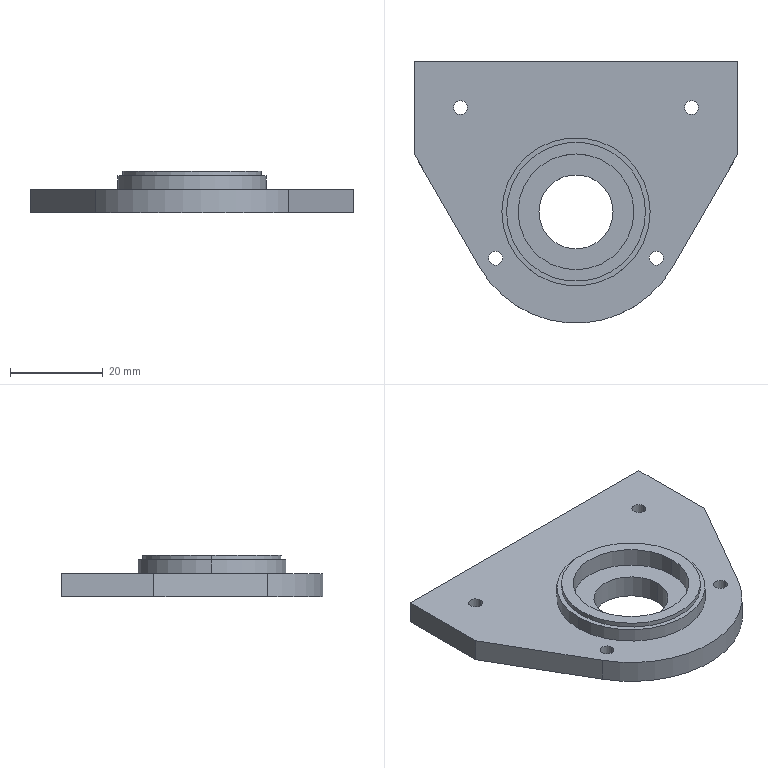Part | SolidWorks | features BaseBody 1 | 1 solid | 39 faces | box 69.859 x 56.5 x 9 mm | volume 15464 mm3 | cylinder 25 | plane 14 | commonest cylinder face diameters 3 x8 5 x8 16 x2 25 x2 30 x2 32 x2
STEP:
#1=CARTESIAN_POINT('',(-22.43,22.5,2.5));
#2=VERTEX_POINT('',#1);
#3=CARTESIAN_POINT('',(-27.43,22.5,2.5));
#4=VERTEX_POINT('',#3);
#5=CARTESIAN_POINT('',(-24.93,22.5,2.5));
#6=DIRECTION('',(0.,0.,1.));
#7=DIRECTION('',(1.,0.,0.));
#8=AXIS2_PLACEMENT_3D('',#5,#6,#7);
#9=CIRCLE('',#8,2.5);
#10=EDGE_CURVE('',#2,#4,#9,.T.);
#11=ORIENTED_EDGE('',*,*,#10,.T.);
#12=CARTESIAN_POINT('',(-27.43,22.5,0.));
#13=VERTEX_POINT('',#12);
#14=CARTESIAN_POINT('',(-27.43,22.5,0.));
#15=DIRECTION('',(0.,0.,-1.));
#16=VECTOR('',#15,1000.);
#17=LINE('',#14,#16);
#18=EDGE_CURVE('',#4,#13,#17,.T.);
#19=ORIENTED_EDGE('',*,*,#18,.T.);
#20=CARTESIAN_POINT('',(-22.43,22.5,0.));
#21=VERTEX_POINT('',#20);
#22=CARTESIAN_POINT('',(-24.93,22.5,0.));
#23=DIRECTION('',(0.,0.,1.));
#24=DIRECTION('',(1.,0.,0.));
#25=AXIS2_PLACEMENT_3D('',#22,#23,#24);
#26=CIRCLE('',#25,2.5);
#27=EDGE_CURVE('',#21,#13,#26,.T.);
#28=ORIENTED_EDGE('',*,*,#27,.F.);
#29=CARTESIAN_POINT('',(-22.43,22.5,0.));
#30=DIRECTION('',(0.,0.,-1.));
#31=VECTOR('',#30,1000.);
#32=LINE('',#29,#31);
#33=EDGE_CURVE('',#2,#21,#32,.T.);
#34=ORIENTED_EDGE('',*,*,#33,.F.);
#35=EDGE_LOOP('',(#11,#19,#28,#34));
#36=FACE_OUTER_BOUND('',#35,.T.);
#37=CARTESIAN_POINT('',(-24.93,22.5,0.));
#38=DIRECTION('',(0.,0.,-1.));
#39=DIRECTION('',(1.,0.,0.));
#40=AXIS2_PLACEMENT_3D('',#37,#38,#39);
#41=CYLINDRICAL_SURFACE('',#40,2.5);
#42=ADVANCED_FACE('',(#36),#41,.F.);
#43=CARTESIAN_POINT('',(-14.821,-10.,2.5));
#44=VERTEX_POINT('',#43);
#45=CARTESIAN_POINT('',(-19.821,-10.,2.5));
#46=VERTEX_POINT('',#45);
#47=CARTESIAN_POINT('',(-17.321,-10.,2.5));
#48=DIRECTION('',(0.,0.,1.));
#49=DIRECTION('',(1.,0.,0.));
#50=AXIS2_PLACEMENT_3D('',#47,#48,#49);
#51=CIRCLE('',#50,2.5);
#52=EDGE_CURVE('',#44,#46,#51,.T.);
#53=ORIENTED_EDGE('',*,*,#52,.T.);
#54=CARTESIAN_POINT('',(-19.821,-10.,0.));
#55=VERTEX_POINT('',#54);
#56=CARTESIAN_POINT('',(-19.821,-10.,0.));
#57=DIRECTION('',(0.,0.,-1.));
#58=VECTOR('',#57,1000.);
#59=LINE('',#56,#58);
#60=EDGE_CURVE('',#46,#55,#59,.T.);
#61=ORIENTED_EDGE('',*,*,#60,.T.);
#62=CARTESIAN_POINT('',(-14.821,-10.,0.));
#63=VERTEX_POINT('',#62);
#64=CARTESIAN_POINT('',(-17.321,-10.,0.));
#65=DIRECTION('',(0.,0.,1.));
#66=DIRECTION('',(1.,0.,0.));
#67=AXIS2_PLACEMENT_3D('',#64,#65,#66);
#68=CIRCLE('',#67,2.5);
#69=EDGE_CURVE('',#63,#55,#68,.T.);
#70=ORIENTED_EDGE('',*,*,#69,.F.);
#71=CARTESIAN_POINT('',(-14.821,-10.,0.));
#72=DIRECTION('',(0.,0.,-1.));
#73=VECTOR('',#72,1000.);
#74=LINE('',#71,#73);
#75=EDGE_CURVE('',#44,#63,#74,.T.);
#76=ORIENTED_EDGE('',*,*,#75,.F.);
#77=EDGE_LOOP('',(#53,#61,#70,#76));
#78=FACE_OUTER_BOUND('',#77,.T.);
#79=CARTESIAN_POINT('',(-17.321,-10.,0.));
#80=DIRECTION('',(0.,0.,-1.));
#81=DIRECTION('',(1.,0.,0.));
#82=AXIS2_PLACEMENT_3D('',#79,#80,#81);
#83=CYLINDRICAL_SURFACE('',#82,2.5);
#84=ADVANCED_FACE('',(#78),#83,.F.);
#85=CARTESIAN_POINT('',(19.821,-10.,2.5));
#86=VERTEX_POINT('',#85);
#87=CARTESIAN_POINT('',(14.821,-10.,2.5));
#88=VERTEX_POINT('',#87);
#89=CARTESIAN_POINT('',(17.321,-10.,2.5));
#90=DIRECTION('',(0.,0.,1.));
#91=DIRECTION('',(1.,0.,0.));
#92=AXIS2_PLACEMENT_3D('',#89,#90,#91);
#93=CIRCLE('',#92,2.5);
#94=EDGE_CURVE('',#86,#88,#93,.T.);
#95=ORIENTED_EDGE('',*,*,#94,.T.);
#96=CARTESIAN_POINT('',(14.821,-10.,0.));
#97=VERTEX_POINT('',#96);
#98=CARTESIAN_POINT('',(14.821,-10.,0.));
#99=DIRECTION('',(0.,0.,-1.));
#100=VECTOR('',#99,1000.);
#101=LINE('',#98,#100);
#102=EDGE_CURVE('',#88,#97,#101,.T.);
#103=ORIENTED_EDGE('',*,*,#102,.T.);
#104=CARTESIAN_POINT('',(19.821,-10.,0.));
#105=VERTEX_POINT('',#104);
#106=CARTESIAN_POINT('',(17.321,-10.,0.));
#107=DIRECTION('',(0.,0.,1.));
#108=DIRECTION('',(1.,0.,0.));
#109=AXIS2_PLACEMENT_3D('',#106,#107,#108);
#110=CIRCLE('',#109,2.5);
#111=EDGE_CURVE('',#105,#97,#110,.T.);
#112=ORIENTED_EDGE('',*,*,#111,.F.);
#113=CARTESIAN_POINT('',(19.821,-10.,0.));
#114=DIRECTION('',(0.,0.,-1.));
#115=VECTOR('',#114,1000.);
#116=LINE('',#113,#115);
#117=EDGE_CURVE('',#86,#105,#116,.T.);
#118=ORIENTED_EDGE('',*,*,#117,.F.);
#119=EDGE_LOOP('',(#95,#103,#112,#118));
#120=FACE_OUTER_BOUND('',#119,.T.);
#121=CARTESIAN_POINT('',(17.321,-10.,0.));
#122=DIRECTION('',(0.,0.,-1.));
#123=DIRECTION('',(1.,0.,0.));
#124=AXIS2_PLACEMENT_3D('',#121,#122,#123);
#125=CYLINDRICAL_SURFACE('',#124,2.5);
#126=ADVANCED_FACE('',(#120),#125,.F.);
#127=CARTESIAN_POINT('',(27.43,22.5,2.5));
#128=VERTEX_POINT('',#127);
#129=CARTESIAN_POINT('',(22.43,22.5,2.5));
#130=VERTEX_POINT('',#129);
#131=CARTESIAN_POINT('',(24.93,22.5,2.5));
#132=DIRECTION('',(0.,0.,1.));
#133=DIRECTION('',(1.,0.,0.));
#134=AXIS2_PLACEMENT_3D('',#131,#132,#133);
#135=CIRCLE('',#134,2.5);
#136=EDGE_CURVE('',#128,#130,#135,.T.);
#137=ORIENTED_EDGE('',*,*,#136,.T.);
#138=CARTESIAN_POINT('',(22.43,22.5,0.));
#139=VERTEX_POINT('',#138);
#140=CARTESIAN_POINT('',(22.43,22.5,0.));
#141=DIRECTION('',(0.,0.,-1.));
#142=VECTOR('',#141,1000.);
#143=LINE('',#140,#142);
#144=EDGE_CURVE('',#130,#139,#143,.T.);
#145=ORIENTED_EDGE('',*,*,#144,.T.);
#146=CARTESIAN_POINT('',(27.43,22.5,0.));
#147=VERTEX_POINT('',#146);
#148=CARTESIAN_POINT('',(24.93,22.5,0.));
#149=DIRECTION('',(0.,0.,1.));
#150=DIRECTION('',(1.,0.,0.));
#151=AXIS2_PLACEMENT_3D('',#148,#149,#150);
#152=CIRCLE('',#151,2.5);
#153=EDGE_CURVE('',#147,#139,#152,.T.);
#154=ORIENTED_EDGE('',*,*,#153,.F.);
#155=CARTESIAN_POINT('',(27.43,22.5,0.));
#156=DIRECTION('',(0.,0.,-1.));
#157=VECTOR('',#156,1000.);
#158=LINE('',#155,#157);
#159=EDGE_CURVE('',#128,#147,#158,.T.);
#160=ORIENTED_EDGE('',*,*,#159,.F.);
#161=EDGE_LOOP('',(#137,#145,#154,#160));
#162=FACE_OUTER_BOUND('',#161,.T.);
#163=CARTESIAN_POINT('',(24.93,22.5,0.));
#164=DIRECTION('',(0.,0.,-1.));
#165=DIRECTION('',(1.,0.,0.));
#166=AXIS2_PLACEMENT_3D('',#163,#164,#165);
#167=CYLINDRICAL_SURFACE('',#166,2.5);
#168=ADVANCED_FACE('',(#162),#167,.F.);
#169=CARTESIAN_POINT('',(23.43,22.5,2.5));
#170=VERTEX_POINT('',#169);
#171=CARTESIAN_POINT('',(26.43,22.5,2.5));
#172=VERTEX_POINT('',#171);
#173=CARTESIAN_POINT('',(24.93,22.5,2.5));
#174=DIRECTION('',(0.,0.,-1.));
#175=DIRECTION('',(-1.,0.,0.));
#176=AXIS2_PLACEMENT_3D('',#173,#174,#175);
#177=CIRCLE('',#176,1.5);
#178=EDGE_CURVE('',#170,#172,#177,.T.);
#179=ORIENTED_EDGE('',*,*,#178,.T.);
#180=CARTESIAN_POINT('',(26.43,22.5,5.));
#181=VERTEX_POINT('',#180);
#182=CARTESIAN_POINT('',(26.43,22.5,5.));
#183=DIRECTION('',(0.,0.,1.));
#184=VECTOR('',#183,1000.);
#185=LINE('',#182,#184);
#186=EDGE_CURVE('',#172,#181,#185,.T.);
#187=ORIENTED_EDGE('',*,*,#186,.T.);
#188=CARTESIAN_POINT('',(23.43,22.5,5.));
#189=VERTEX_POINT('',#188);
#190=CARTESIAN_POINT('',(24.93,22.5,5.));
#191=DIRECTION('',(0.,0.,-1.));
#192=DIRECTION('',(-1.,0.,0.));
#193=AXIS2_PLACEMENT_3D('',#190,#191,#192);
#194=CIRCLE('',#193,1.5);
#195=EDGE_CURVE('',#189,#181,#194,.T.);
#196=ORIENTED_EDGE('',*,*,#195,.F.);
#197=CARTESIAN_POINT('',(23.43,22.5,5.));
#198=DIRECTION('',(0.,0.,1.));
#199=VECTOR('',#198,1000.);
#200=LINE('',#197,#199);
#201=EDGE_CURVE('',#170,#189,#200,.T.);
#202=ORIENTED_EDGE('',*,*,#201,.F.);
#203=EDGE_LOOP('',(#179,#187,#196,#202));
#204=FACE_OUTER_BOUND('',#203,.T.);
#205=CARTESIAN_POINT('',(24.93,22.5,5.));
#206=DIRECTION('',(0.,0.,1.));
#207=DIRECTION('',(-1.,0.,0.));
#208=AXIS2_PLACEMENT_3D('',#205,#206,#207);
#209=CYLINDRICAL_SURFACE('',#208,1.5);
#210=ADVANCED_FACE('',(#204),#209,.F.);
#211=CARTESIAN_POINT('',(15.821,-10.,2.5));
#212=VERTEX_POINT('',#211);
#213=CARTESIAN_POINT('',(18.821,-10.,2.5));
#214=VERTEX_POINT('',#213);
#215=CARTESIAN_POINT('',(17.321,-10.,2.5));
#216=DIRECTION('',(0.,0.,-1.));
#217=DIRECTION('',(-1.,0.,0.));
#218=AXIS2_PLACEMENT_3D('',#215,#216,#217);
#219=CIRCLE('',#218,1.5);
#220=EDGE_CURVE('',#212,#214,#219,.T.);
#221=ORIENTED_EDGE('',*,*,#220,.T.);
#222=CARTESIAN_POINT('',(18.821,-10.,5.));
#223=VERTEX_POINT('',#222);
#224=CARTESIAN_POINT('',(18.821,-10.,5.));
#225=DIRECTION('',(0.,0.,1.));
#226=VECTOR('',#225,1000.);
#227=LINE('',#224,#226);
#228=EDGE_CURVE('',#214,#223,#227,.T.);
#229=ORIENTED_EDGE('',*,*,#228,.T.);
#230=CARTESIAN_POINT('',(15.821,-10.,5.));
#231=VERTEX_POINT('',#230);
#232=CARTESIAN_POINT('',(17.321,-10.,5.));
#233=DIRECTION('',(0.,0.,-1.));
#234=DIRECTION('',(-1.,0.,0.));
#235=AXIS2_PLACEMENT_3D('',#232,#233,#234);
#236=CIRCLE('',#235,1.5);
#237=EDGE_CURVE('',#231,#223,#236,.T.);
#238=ORIENTED_EDGE('',*,*,#237,.F.);
#239=CARTESIAN_POINT('',(15.821,-10.,5.));
#240=DIRECTION('',(0.,0.,1.));
#241=VECTOR('',#240,1000.);
#242=LINE('',#239,#241);
#243=EDGE_CURVE('',#212,#231,#242,.T.);
#244=ORIENTED_EDGE('',*,*,#243,.F.);
#245=EDGE_LOOP('',(#221,#229,#238,#244));
#246=FACE_OUTER_BOUND('',#245,.T.);
#247=CARTESIAN_POINT('',(17.321,-10.,5.));
#248=DIRECTION('',(0.,0.,1.));
#249=DIRECTION('',(-1.,0.,0.));
#250=AXIS2_PLACEMENT_3D('',#247,#248,#249);
#251=CYLINDRICAL_SURFACE('',#250,1.5);
#252=ADVANCED_FACE('',(#246),#251,.F.);
#253=CARTESIAN_POINT('',(-18.821,-10.,2.5));
#254=VERTEX_POINT('',#253);
#255=CARTESIAN_POINT('',(-15.821,-10.,2.5));
#256=VERTEX_POINT('',#255);
#257=CARTESIAN_POINT('',(-17.321,-10.,2.5));
#258=DIRECTION('',(0.,0.,-1.));
#259=DIRECTION('',(-1.,0.,0.));
#260=AXIS2_PLACEMENT_3D('',#257,#258,#259);
#261=CIRCLE('',#260,1.5);
#262=EDGE_CURVE('',#254,#256,#261,.T.);
#263=ORIENTED_EDGE('',*,*,#262,.T.);
#264=CARTESIAN_POINT('',(-15.821,-10.,5.));
#265=VERTEX_POINT('',#264);
#266=CARTESIAN_POINT('',(-15.821,-10.,5.));
#267=DIRECTION('',(0.,0.,1.));
#268=VECTOR('',#267,1000.);
#269=LINE('',#266,#268);
#270=EDGE_CURVE('',#256,#265,#269,.T.);
#271=ORIENTED_EDGE('',*,*,#270,.T.);
#272=CARTESIAN_POINT('',(-18.821,-10.,5.));
#273=VERTEX_POINT('',#272);
#274=CARTESIAN_POINT('',(-17.321,-10.,5.));
#275=DIRECTION('',(0.,0.,-1.));
#276=DIRECTION('',(-1.,0.,0.));
#277=AXIS2_PLACEMENT_3D('',#274,#275,#276);
#278=CIRCLE('',#277,1.5);
#279=EDGE_CURVE('',#273,#265,#278,.T.);
#280=ORIENTED_EDGE('',*,*,#279,.F.);
#281=CARTESIAN_POINT('',(-18.821,-10.,5.));
#282=DIRECTION('',(0.,0.,1.));
#283=VECTOR('',#282,1000.);
#284=LINE('',#281,#283);
#285=EDGE_CURVE('',#254,#273,#284,.T.);
#286=ORIENTED_EDGE('',*,*,#285,.F.);
#287=EDGE_LOOP('',(#263,#271,#280,#286));
#288=FACE_OUTER_BOUND('',#287,.T.);
#289=CARTESIAN_POINT('',(-17.321,-10.,5.));
#290=DIRECTION('',(0.,0.,1.));
#291=DIRECTION('',(-1.,0.,0.));
#292=AXIS2_PLACEMENT_3D('',#289,#290,#291);
#293=CYLINDRICAL_SURFACE('',#292,1.5);
#294=ADVANCED_FACE('',(#288),#293,.F.);
#295=CARTESIAN_POINT('',(-26.43,22.5,2.5));
#296=VERTEX_POINT('',#295);
#297=CARTESIAN_POINT('',(-23.43,22.5,2.5));
#298=VERTEX_POINT('',#297);
#299=CARTESIAN_POINT('',(-24.93,22.5,2.5));
#300=DIRECTION('',(0.,0.,-1.));
#301=DIRECTION('',(-1.,0.,0.));
#302=AXIS2_PLACEMENT_3D('',#299,#300,#301);
#303=CIRCLE('',#302,1.5);
#304=EDGE_CURVE('',#296,#298,#303,.T.);
#305=ORIENTED_EDGE('',*,*,#304,.T.);
#306=CARTESIAN_POINT('',(-23.43,22.5,5.));
#307=VERTEX_POINT('',#306);
#308=CARTESIAN_POINT('',(-23.43,22.5,5.));
#309=DIRECTION('',(0.,0.,1.));
#310=VECTOR('',#309,1000.);
#311=LINE('',#308,#310);
#312=EDGE_CURVE('',#298,#307,#311,.T.);
#313=ORIENTED_EDGE('',*,*,#312,.T.);
#314=CARTESIAN_POINT('',(-26.43,22.5,5.));
#315=VERTEX_POINT('',#314);
#316=CARTESIAN_POINT('',(-24.93,22.5,5.));
#317=DIRECTION('',(0.,0.,-1.));
#318=DIRECTION('',(-1.,0.,0.));
#319=AXIS2_PLACEMENT_3D('',#316,#317,#318);
#320=CIRCLE('',#319,1.5);
#321=EDGE_CURVE('',#315,#307,#320,.T.);
#322=ORIENTED_EDGE('',*,*,#321,.F.);
#323=CARTESIAN_POINT('',(-26.43,22.5,5.));
#324=DIRECTION('',(0.,0.,1.));
#325=VECTOR('',#324,1000.);
#326=LINE('',#323,#325);
#327=EDGE_CURVE('',#296,#315,#326,.T.);
#328=ORIENTED_EDGE('',*,*,#327,.F.);
#329=EDGE_LOOP('',(#305,#313,#322,#328));
#330=FACE_OUTER_BOUND('',#329,.T.);
#331=CARTESIAN_POINT('',(-24.93,22.5,5.));
#332=DIRECTION('',(0.,0.,1.));
#333=DIRECTION('',(-1.,0.,0.));
#334=AXIS2_PLACEMENT_3D('',#331,#332,#333);
#335=CYLINDRICAL_SURFACE('',#334,1.5);
#336=ADVANCED_FACE('',(#330),#335,.F.);
#337=CARTESIAN_POINT('',(8.,0.,0.));
#338=VERTEX_POINT('',#337);
#339=CARTESIAN_POINT('',(-8.,0.,0.));
#340=VERTEX_POINT('',#339);
#341=CARTESIAN_POINT('',(0.,0.,0.));
#342=DIRECTION('',(0.,0.,1.));
#343=DIRECTION('',(-1.,0.,0.));
#344=AXIS2_PLACEMENT_3D('',#341,#342,#343);
#345=CIRCLE('',#344,8.);
#346=EDGE_CURVE('',#338,#340,#345,.T.);
#347=ORIENTED_EDGE('',*,*,#346,.F.);
#348=CARTESIAN_POINT('',(8.,0.,5.));
#349=VERTEX_POINT('',#348);
#350=CARTESIAN_POINT('',(8.,0.,5.));
#351=DIRECTION('',(0.,0.,1.));
#352=VECTOR('',#351,1000.);
#353=LINE('',#350,#352);
#354=EDGE_CURVE('',#338,#349,#353,.T.);
#355=ORIENTED_EDGE('',*,*,#354,.T.);
#356=CARTESIAN_POINT('',(-8.,0.,5.));
#357=VERTEX_POINT('',#356);
#358=CARTESIAN_POINT('',(0.,0.,5.));
#359=DIRECTION('',(0.,0.,-1.));
#360=DIRECTION('',(-1.,0.,0.));
#361=AXIS2_PLACEMENT_3D('',#358,#359,#360);
#362=CIRCLE('',#361,8.);
#363=EDGE_CURVE('',#357,#349,#362,.T.);
#364=ORIENTED_EDGE('',*,*,#363,.F.);
#365=CARTESIAN_POINT('',(-8.,0.,5.));
#366=DIRECTION('',(0.,0.,1.));
#367=VECTOR('',#366,1000.);
#368=LINE('',#365,#367);
#369=EDGE_CURVE('',#340,#357,#368,.T.);
#370=ORIENTED_EDGE('',*,*,#369,.F.);
#371=EDGE_LOOP('',(#347,#355,#364,#370));
#372=FACE_OUTER_BOUND('',#371,.T.);
#373=CARTESIAN_POINT('',(0.,0.,5.));
#374=DIRECTION('',(0.,0.,1.));
#375=DIRECTION('',(-1.,0.,0.));
#376=AXIS2_PLACEMENT_3D('',#373,#374,#375);
#377=CYLINDRICAL_SURFACE('',#376,8.);
#378=ADVANCED_FACE('',(#372),#377,.F.);
#379=CARTESIAN_POINT('',(-15.,0.,8.));
#380=VERTEX_POINT('',#379);
#381=CARTESIAN_POINT('',(15.,0.,8.));
#382=VERTEX_POINT('',#381);
#383=CARTESIAN_POINT('',(0.,0.,8.));
#384=DIRECTION('',(0.,0.,1.));
#385=DIRECTION('',(-1.,0.,0.));
#386=AXIS2_PLACEMENT_3D('',#383,#384,#385);
#387=CIRCLE('',#386,15.);
#388=EDGE_CURVE('',#380,#382,#387,.T.);
#389=ORIENTED_EDGE('',*,*,#388,.T.);
#390=CARTESIAN_POINT('',(15.,0.,9.));
#391=VERTEX_POINT('',#390);
#392=CARTESIAN_POINT('',(15.,0.,9.));
#393=DIRECTION('',(0.,0.,1.));
#394=VECTOR('',#393,1000.);
#395=LINE('',#392,#394);
#396=EDGE_CURVE('',#382,#391,#395,.T.);
#397=ORIENTED_EDGE('',*,*,#396,.T.);
#398=CARTESIAN_POINT('',(-15.,0.,9.));
#399=VERTEX_POINT('',#398);
#400=CARTESIAN_POINT('',(0.,0.,9.));
#401=DIRECTION('',(0.,0.,1.));
#402=DIRECTION('',(-1.,0.,0.));
#403=AXIS2_PLACEMENT_3D('',#400,#401,#402);
#404=CIRCLE('',#403,15.);
#405=EDGE_CURVE('',#399,#391,#404,.T.);
#406=ORIENTED_EDGE('',*,*,#405,.F.);
#407=CARTESIAN_POINT('',(-15.,0.,9.));
#408=DIRECTION('',(0.,0.,1.));
#409=VECTOR('',#408,1000.);
#410=LINE('',#407,#409);
#411=EDGE_CURVE('',#380,#399,#410,.T.);
#412=ORIENTED_EDGE('',*,*,#411,.F.);
#413=EDGE_LOOP('',(#389,#397,#406,#412));
#414=FACE_OUTER_BOUND('',#413,.T.);
#415=CARTESIAN_POINT('',(0.,0.,9.));
#416=DIRECTION('',(0.,0.,1.));
#417=DIRECTION('',(-1.,0.,0.));
#418=AXIS2_PLACEMENT_3D('',#415,#416,#417);
#419=CYLINDRICAL_SURFACE('',#418,15.);
#420=ADVANCED_FACE('',(#414),#419,.T.);
#421=CARTESIAN_POINT('',(12.5,0.,9.));
#422=VERTEX_POINT('',#421);
#423=CARTESIAN_POINT('',(-12.5,0.,9.));
#424=VERTEX_POINT('',#423);
#425=CARTESIAN_POINT('',(0.,0.,9.));
#426=DIRECTION('',(0.,0.,-1.));
#427=DIRECTION('',(-1.,0.,0.));
#428=AXIS2_PLACEMENT_3D('',#425,#426,#427);
#429=CIRCLE('',#428,12.5);
#430=EDGE_CURVE('',#422,#424,#429,.T.);
#431=ORIENTED_EDGE('',*,*,#430,.F.);
#432=CARTESIAN_POINT('',(12.5,0.,5.));
#433=VERTEX_POINT('',#432);
#434=CARTESIAN_POINT('',(12.5,0.,5.));
#435=DIRECTION('',(0.,0.,-1.));
#436=VECTOR('',#435,1000.);
#437=LINE('',#434,#436);
#438=EDGE_CURVE('',#422,#433,#437,.T.);
#439=ORIENTED_EDGE('',*,*,#438,.T.);
#440=CARTESIAN_POINT('',(-12.5,0.,5.));
#441=VERTEX_POINT('',#440);
#442=CARTESIAN_POINT('',(0.,0.,5.));
#443=DIRECTION('',(0.,0.,1.));
#444=DIRECTION('',(-1.,0.,0.));
#445=AXIS2_PLACEMENT_3D('',#442,#443,#444);
#446=CIRCLE('',#445,12.5);
#447=EDGE_CURVE('',#441,#433,#446,.T.);
#448=ORIENTED_EDGE('',*,*,#447,.F.);
#449=CARTESIAN_POINT('',(-12.5,0.,5.));
#450=DIRECTION('',(0.,0.,-1.));
#451=VECTOR('',#450,1000.);
#452=LINE('',#449,#451);
#453=EDGE_CURVE('',#424,#441,#452,.T.);
#454=ORIENTED_EDGE('',*,*,#453,.F.);
#455=EDGE_LOOP('',(#431,#439,#448,#454));
#456=FACE_OUTER_BOUND('',#455,.T.);
#457=CARTESIAN_POINT('',(0.,0.,5.));
#458=DIRECTION('',(0.,0.,-1.));
#459=DIRECTION('',(-1.,0.,0.));
#460=AXIS2_PLACEMENT_3D('',#457,#458,#459);
#461=CYLINDRICAL_SURFACE('',#460,12.5);
#462=ADVANCED_FACE('',(#456),#461,.F.);
#463=CARTESIAN_POINT('',(-16.,0.,8.));
#464=VERTEX_POINT('',#463);
#465=CARTESIAN_POINT('',(16.,0.,8.));
#466=VERTEX_POINT('',#465);
#467=CARTESIAN_POINT('',(0.,0.,8.));
#468=DIRECTION('',(0.,0.,-1.));
#469=DIRECTION('',(-1.,0.,0.));
#470=AXIS2_PLACEMENT_3D('',#467,#468,#469);
#471=CIRCLE('',#470,16.);
#472=EDGE_CURVE('',#464,#466,#471,.T.);
#473=ORIENTED_EDGE('',*,*,#472,.T.);
#474=CARTESIAN_POINT('',(16.,0.,5.));
#475=VERTEX_POINT('',#474);
#476=CARTESIAN_POINT('',(16.,0.,5.));
#477=DIRECTION('',(0.,0.,-1.));
#478=VECTOR('',#477,1000.);
#479=LINE('',#476,#478);
#480=EDGE_CURVE('',#466,#475,#479,.T.);
#481=ORIENTED_EDGE('',*,*,#480,.T.);
#482=CARTESIAN_POINT('',(-16.,0.,5.));
#483=VERTEX_POINT('',#482);
#484=CARTESIAN_POINT('',(0.,0.,5.));
#485=DIRECTION('',(0.,0.,-1.));
#486=DIRECTION('',(-1.,0.,0.));
#487=AXIS2_PLACEMENT_3D('',#484,#485,#486);
#488=CIRCLE('',#487,16.);
#489=EDGE_CURVE('',#483,#475,#488,.T.);
#490=ORIENTED_EDGE('',*,*,#489,.F.);
#491=CARTESIAN_POINT('',(-16.,0.,5.));
#492=DIRECTION('',(0.,0.,-1.));
#493=VECTOR('',#492,1000.);
#494=LINE('',#491,#493);
#495=EDGE_CURVE('',#464,#483,#494,.T.);
#496=ORIENTED_EDGE('',*,*,#495,.F.);
#497=EDGE_LOOP('',(#473,#481,#490,#496));
#498=FACE_OUTER_BOUND('',#497,.T.);
#499=CARTESIAN_POINT('',(0.,0.,5.));
#500=DIRECTION('',(0.,0.,-1.));
#501=DIRECTION('',(-1.,0.,0.));
#502=AXIS2_PLACEMENT_3D('',#499,#500,#501);
#503=CYLINDRICAL_SURFACE('',#502,16.);
#504=ADVANCED_FACE('',(#498),#503,.T.);
#505=ORIENTED_EDGE('',*,*,#304,.F.);
#506=CARTESIAN_POINT('',(-24.93,22.5,2.5));
#507=DIRECTION('',(0.,0.,-1.));
#508=DIRECTION('',(-1.,0.,0.));
#509=AXIS2_PLACEMENT_3D('',#506,#507,#508);
#510=CIRCLE('',#509,1.5);
#511=EDGE_CURVE('',#298,#296,#510,.T.);
#512=ORIENTED_EDGE('',*,*,#511,.F.);
#513=EDGE_LOOP('',(#505,#512));
#514=FACE_BOUND('',#513,.T.);
#515=ORIENTED_EDGE('',*,*,#10,.F.);
#516=CARTESIAN_POINT('',(-24.93,22.5,2.5));
#517=DIRECTION('',(0.,0.,1.));
#518=DIRECTION('',(1.,0.,0.));
#519=AXIS2_PLACEMENT_3D('',#516,#517,#518);
#520=CIRCLE('',#519,2.5);
#521=EDGE_CURVE('',#4,#2,#520,.T.);
#522=ORIENTED_EDGE('',*,*,#521,.F.);
#523=EDGE_LOOP('',(#515,#522));
#524=FACE_OUTER_BOUND('',#523,.T.);
#525=CARTESIAN_POINT('',(-24.93,22.5,2.5));
#526=DIRECTION('',(0.,0.,1.));
#527=DIRECTION('',(1.,0.,0.));
#528=AXIS2_PLACEMENT_3D('',#525,#526,#527);
#529=PLANE('',#528);
#530=ADVANCED_FACE('',(#514,#524),#529,.F.);
#531=ORIENTED_EDGE('',*,*,#262,.F.);
#532=CARTESIAN_POINT('',(-17.321,-10.,2.5));
#533=DIRECTION('',(0.,0.,-1.));
#534=DIRECTION('',(-1.,0.,0.));
#535=AXIS2_PLACEMENT_3D('',#532,#533,#534);
#536=CIRCLE('',#535,1.5);
#537=EDGE_CURVE('',#256,#254,#536,.T.);
#538=ORIENTED_EDGE('',*,*,#537,.F.);
#539=EDGE_LOOP('',(#531,#538));
#540=FACE_BOUND('',#539,.T.);
#541=ORIENTED_EDGE('',*,*,#52,.F.);
#542=CARTESIAN_POINT('',(-17.321,-10.,2.5));
#543=DIRECTION('',(0.,0.,1.));
#544=DIRECTION('',(1.,0.,0.));
#545=AXIS2_PLACEMENT_3D('',#542,#543,#544);
#546=CIRCLE('',#545,2.5);
#547=EDGE_CURVE('',#46,#44,#546,.T.);
#548=ORIENTED_EDGE('',*,*,#547,.F.);
#549=EDGE_LOOP('',(#541,#548));
#550=FACE_OUTER_BOUND('',#549,.T.);
#551=CARTESIAN_POINT('',(-17.321,-10.,2.5));
#552=DIRECTION('',(0.,0.,1.));
#553=DIRECTION('',(1.,0.,0.));
#554=AXIS2_PLACEMENT_3D('',#551,#552,#553);
#555=PLANE('',#554);
#556=ADVANCED_FACE('',(#540,#550),#555,.F.);
#557=ORIENTED_EDGE('',*,*,#220,.F.);
#558=CARTESIAN_POINT('',(17.321,-10.,2.5));
#559=DIRECTION('',(0.,0.,-1.));
#560=DIRECTION('',(-1.,0.,0.));
#561=AXIS2_PLACEMENT_3D('',#558,#559,#560);
#562=CIRCLE('',#561,1.5);
#563=EDGE_CURVE('',#214,#212,#562,.T.);
#564=ORIENTED_EDGE('',*,*,#563,.F.);
#565=EDGE_LOOP('',(#557,#564));
#566=FACE_BOUND('',#565,.T.);
#567=ORIENTED_EDGE('',*,*,#94,.F.);
#568=CARTESIAN_POINT('',(17.321,-10.,2.5));
#569=DIRECTION('',(0.,0.,1.));
#570=DIRECTION('',(1.,0.,0.));
#571=AXIS2_PLACEMENT_3D('',#568,#569,#570);
#572=CIRCLE('',#571,2.5);
#573=EDGE_CURVE('',#88,#86,#572,.T.);
#574=ORIENTED_EDGE('',*,*,#573,.F.);
#575=EDGE_LOOP('',(#567,#574));
#576=FACE_OUTER_BOUND('',#575,.T.);
#577=CARTESIAN_POINT('',(17.321,-10.,2.5));
#578=DIRECTION('',(0.,0.,1.));
#579=DIRECTION('',(1.,0.,0.));
#580=AXIS2_PLACEMENT_3D('',#577,#578,#579);
#581=PLANE('',#580);
#582=ADVANCED_FACE('',(#566,#576),#581,.F.);
#583=ORIENTED_EDGE('',*,*,#178,.F.);
#584=CARTESIAN_POINT('',(24.93,22.5,2.5));
#585=DIRECTION('',(0.,0.,-1.));
#586=DIRECTION('',(-1.,0.,0.));
#587=AXIS2_PLACEMENT_3D('',#584,#585,#586);
#588=CIRCLE('',#587,1.5);
#589=EDGE_CURVE('',#172,#170,#588,.T.);
#590=ORIENTED_EDGE('',*,*,#589,.F.);
#591=EDGE_LOOP('',(#583,#590));
#592=FACE_BOUND('',#591,.T.);
#593=ORIENTED_EDGE('',*,*,#136,.F.);
#594=CARTESIAN_POINT('',(24.93,22.5,2.5));
#595=DIRECTION('',(0.,0.,1.));
#596=DIRECTION('',(1.,0.,0.));
#597=AXIS2_PLACEMENT_3D('',#594,#595,#596);
#598=CIRCLE('',#597,2.5);
#599=EDGE_CURVE('',#130,#128,#598,.T.);
#600=ORIENTED_EDGE('',*,*,#599,.F.);
#601=EDGE_LOOP('',(#593,#600));
#602=FACE_OUTER_BOUND('',#601,.T.);
#603=CARTESIAN_POINT('',(24.93,22.5,2.5));
#604=DIRECTION('',(0.,0.,1.));
#605=DIRECTION('',(1.,0.,0.));
#606=AXIS2_PLACEMENT_3D('',#603,#604,#605);
#607=PLANE('',#606);
#608=ADVANCED_FACE('',(#592,#602),#607,.F.);
#609=ORIENTED_EDGE('',*,*,#388,.F.);
#610=CARTESIAN_POINT('',(0.,0.,8.));
#611=DIRECTION('',(0.,0.,1.));
#612=DIRECTION('',(-1.,0.,0.));
#613=AXIS2_PLACEMENT_3D('',#610,#611,#612);
#614=CIRCLE('',#613,15.);
#615=EDGE_CURVE('',#382,#380,#614,.T.);
#616=ORIENTED_EDGE('',*,*,#615,.F.);
#617=EDGE_LOOP('',(#609,#616));
#618=FACE_BOUND('',#617,.T.);
#619=ORIENTED_EDGE('',*,*,#472,.F.);
#620=CARTESIAN_POINT('',(0.,0.,8.));
#621=DIRECTION('',(0.,0.,-1.));
#622=DIRECTION('',(-1.,0.,0.));
#623=AXIS2_PLACEMENT_3D('',#620,#621,#622);
#624=CIRCLE('',#623,16.);
#625=EDGE_CURVE('',#466,#464,#624,.T.);
#626=ORIENTED_EDGE('',*,*,#625,.F.);
#627=EDGE_LOOP('',(#619,#626));
#628=FACE_OUTER_BOUND('',#627,.T.);
#629=CARTESIAN_POINT('',(0.,0.,8.));
#630=DIRECTION('',(0.,0.,1.));
#631=DIRECTION('',(1.,0.,0.));
#632=AXIS2_PLACEMENT_3D('',#629,#630,#631);
#633=PLANE('',#632);
#634=ADVANCED_FACE('',(#618,#628),#633,.T.);
#635=CARTESIAN_POINT('',(0.,0.,9.));
#636=DIRECTION('',(0.,0.,-1.));
#637=DIRECTION('',(-1.,0.,0.));
#638=AXIS2_PLACEMENT_3D('',#635,#636,#637);
#639=CIRCLE('',#638,12.5);
#640=EDGE_CURVE('',#424,#422,#639,.T.);
#641=ORIENTED_EDGE('',*,*,#640,.T.);
#642=ORIENTED_EDGE('',*,*,#430,.T.);
#643=EDGE_LOOP('',(#641,#642));
#644=FACE_BOUND('',#643,.T.);
#645=ORIENTED_EDGE('',*,*,#405,.T.);
#646=CARTESIAN_POINT('',(0.,0.,9.));
#647=DIRECTION('',(0.,0.,1.));
#648=DIRECTION('',(-1.,0.,0.));
#649=AXIS2_PLACEMENT_3D('',#646,#647,#648);
#650=CIRCLE('',#649,15.);
#651=EDGE_CURVE('',#391,#399,#650,.T.);
#652=ORIENTED_EDGE('',*,*,#651,.T.);
#653=EDGE_LOOP('',(#645,#652));
#654=FACE_OUTER_BOUND('',#653,.T.);
#655=CARTESIAN_POINT('',(0.,0.,9.));
#656=DIRECTION('',(0.,0.,1.));
#657=DIRECTION('',(1.,0.,0.));
#658=AXIS2_PLACEMENT_3D('',#655,#656,#657);
#659=PLANE('',#658);
#660=ADVANCED_FACE('',(#644,#654),#659,.T.);
#661=ORIENTED_EDGE('',*,*,#195,.T.);
#662=CARTESIAN_POINT('',(24.93,22.5,5.));
#663=DIRECTION('',(0.,0.,-1.));
#664=DIRECTION('',(-1.,0.,0.));
#665=AXIS2_PLACEMENT_3D('',#662,#663,#664);
#666=CIRCLE('',#665,1.5);
#667=EDGE_CURVE('',#181,#189,#666,.T.);
#668=ORIENTED_EDGE('',*,*,#667,.T.);
#669=EDGE_LOOP('',(#661,#668));
#670=FACE_BOUND('',#669,.T.);
#671=ORIENTED_EDGE('',*,*,#237,.T.);
#672=CARTESIAN_POINT('',(17.321,-10.,5.));
#673=DIRECTION('',(0.,0.,-1.));
#674=DIRECTION('',(-1.,0.,0.));
#675=AXIS2_PLACEMENT_3D('',#672,#673,#674);
#676=CIRCLE('',#675,1.5);
#677=EDGE_CURVE('',#223,#231,#676,.T.);
#678=ORIENTED_EDGE('',*,*,#677,.T.);
#679=EDGE_LOOP('',(#671,#678));
#680=FACE_BOUND('',#679,.T.);
#681=ORIENTED_EDGE('',*,*,#279,.T.);
#682=CARTESIAN_POINT('',(-17.321,-10.,5.));
#683=DIRECTION('',(0.,0.,-1.));
#684=DIRECTION('',(-1.,0.,0.));
#685=AXIS2_PLACEMENT_3D('',#682,#683,#684);
#686=CIRCLE('',#685,1.5);
#687=EDGE_CURVE('',#265,#273,#686,.T.);
#688=ORIENTED_EDGE('',*,*,#687,.T.);
#689=EDGE_LOOP('',(#681,#688));
#690=FACE_BOUND('',#689,.T.);
#691=ORIENTED_EDGE('',*,*,#321,.T.);
#692=CARTESIAN_POINT('',(-24.93,22.5,5.));
#693=DIRECTION('',(0.,0.,-1.));
#694=DIRECTION('',(-1.,0.,0.));
#695=AXIS2_PLACEMENT_3D('',#692,#693,#694);
#696=CIRCLE('',#695,1.5);
#697=EDGE_CURVE('',#307,#315,#696,.T.);
#698=ORIENTED_EDGE('',*,*,#697,.T.);
#699=EDGE_LOOP('',(#691,#698));
#700=FACE_BOUND('',#699,.T.);
#701=ORIENTED_EDGE('',*,*,#489,.T.);
#702=CARTESIAN_POINT('',(0.,0.,5.));
#703=DIRECTION('',(0.,0.,-1.));
#704=DIRECTION('',(-1.,0.,0.));
#705=AXIS2_PLACEMENT_3D('',#702,#703,#704);
#706=CIRCLE('',#705,16.);
#707=EDGE_CURVE('',#475,#483,#706,.T.);
#708=ORIENTED_EDGE('',*,*,#707,.T.);
#709=EDGE_LOOP('',(#701,#708));
#710=FACE_BOUND('',#709,.T.);
#711=CARTESIAN_POINT('',(20.785,-12.,5.));
#712=VERTEX_POINT('',#711);
#713=CARTESIAN_POINT('',(34.93,12.5,5.));
#714=VERTEX_POINT('',#713);
#715=CARTESIAN_POINT('',(20.785,-12.,5.));
#716=DIRECTION('',(0.5,0.866,0.));
#717=VECTOR('',#716,1000.);
#718=LINE('',#715,#717);
#719=EDGE_CURVE('',#712,#714,#718,.T.);
#720=ORIENTED_EDGE('',*,*,#719,.T.);
#721=CARTESIAN_POINT('',(34.93,32.5,5.));
#722=VERTEX_POINT('',#721);
#723=CARTESIAN_POINT('',(34.93,12.5,5.));
#724=DIRECTION('',(0.,1.,0.));
#725=VECTOR('',#724,1000.);
#726=LINE('',#723,#725);
#727=EDGE_CURVE('',#714,#722,#726,.T.);
#728=ORIENTED_EDGE('',*,*,#727,.T.);
#729=CARTESIAN_POINT('',(-34.93,32.5,5.));
#730=VERTEX_POINT('',#729);
#731=CARTESIAN_POINT('',(34.93,32.5,5.));
#732=DIRECTION('',(-1.,0.,0.));
#733=VECTOR('',#732,1000.);
#734=LINE('',#731,#733);
#735=EDGE_CURVE('',#722,#730,#734,.T.);
#736=ORIENTED_EDGE('',*,*,#735,.T.);
#737=CARTESIAN_POINT('',(-34.93,12.5,5.));
#738=VERTEX_POINT('',#737);
#739=CARTESIAN_POINT('',(-34.93,32.5,5.));
#740=DIRECTION('',(0.,-1.,0.));
#741=VECTOR('',#740,1000.);
#742=LINE('',#739,#741);
#743=EDGE_CURVE('',#730,#738,#742,.T.);
#744=ORIENTED_EDGE('',*,*,#743,.T.);
#745=CARTESIAN_POINT('',(-20.785,-12.,5.));
#746=VERTEX_POINT('',#745);
#747=CARTESIAN_POINT('',(-34.93,12.5,5.));
#748=DIRECTION('',(0.5,-0.866,0.));
#749=VECTOR('',#748,1000.);
#750=LINE('',#747,#749);
#751=EDGE_CURVE('',#738,#746,#750,.T.);
#752=ORIENTED_EDGE('',*,*,#751,.T.);
#753=CARTESIAN_POINT('',(0.,0.,5.));
#754=DIRECTION('',(0.,0.,1.));
#755=DIRECTION('',(1.,0.,0.));
#756=AXIS2_PLACEMENT_3D('',#753,#754,#755);
#757=CIRCLE('',#756,24.);
#758=EDGE_CURVE('',#746,#712,#757,.T.);
#759=ORIENTED_EDGE('',*,*,#758,.T.);
#760=EDGE_LOOP('',(#720,#728,#736,#744,#752,#759));
#761=FACE_OUTER_BOUND('',#760,.T.);
#762=CARTESIAN_POINT('',(0.,16.262,5.));
#763=DIRECTION('',(0.,0.,1.));
#764=DIRECTION('',(1.,0.,0.));
#765=AXIS2_PLACEMENT_3D('',#762,#763,#764);
#766=PLANE('',#765);
#767=ADVANCED_FACE('',(#670,#680,#690,#700,#710,#761),#766,.T.);
#768=CARTESIAN_POINT('',(-20.785,-12.,0.));
#769=VERTEX_POINT('',#768);
#770=CARTESIAN_POINT('',(-20.785,-12.,0.));
#771=DIRECTION('',(0.,0.,1.));
#772=VECTOR('',#771,1000.);
#773=LINE('',#770,#772);
#774=EDGE_CURVE('',#769,#746,#773,.T.);
#775=ORIENTED_EDGE('',*,*,#774,.F.);
#776=CARTESIAN_POINT('',(20.785,-12.,0.));
#777=VERTEX_POINT('',#776);
#778=CARTESIAN_POINT('',(0.,0.,0.));
#779=DIRECTION('',(0.,0.,1.));
#780=DIRECTION('',(1.,0.,0.));
#781=AXIS2_PLACEMENT_3D('',#778,#779,#780);
#782=CIRCLE('',#781,24.);
#783=EDGE_CURVE('',#769,#777,#782,.T.);
#784=ORIENTED_EDGE('',*,*,#783,.T.);
#785=CARTESIAN_POINT('',(20.785,-12.,0.));
#786=DIRECTION('',(0.,0.,1.));
#787=VECTOR('',#786,1000.);
#788=LINE('',#785,#787);
#789=EDGE_CURVE('',#777,#712,#788,.T.);
#790=ORIENTED_EDGE('',*,*,#789,.T.);
#791=ORIENTED_EDGE('',*,*,#758,.F.);
#792=EDGE_LOOP('',(#775,#784,#790,#791));
#793=FACE_OUTER_BOUND('',#792,.T.);
#794=CARTESIAN_POINT('',(0.,0.,0.));
#795=DIRECTION('',(0.,0.,-1.));
#796=DIRECTION('',(1.,0.,0.));
#797=AXIS2_PLACEMENT_3D('',#794,#795,#796);
#798=CYLINDRICAL_SURFACE('',#797,24.);
#799=ADVANCED_FACE('',(#793),#798,.T.);
#800=CARTESIAN_POINT('',(-34.93,12.5,0.));
#801=VERTEX_POINT('',#800);
#802=CARTESIAN_POINT('',(-34.93,12.5,0.));
#803=DIRECTION('',(0.5,-0.866,0.));
#804=VECTOR('',#803,1000.);
#805=LINE('',#802,#804);
#806=EDGE_CURVE('',#801,#769,#805,.T.);
#807=ORIENTED_EDGE('',*,*,#806,.T.);
#808=ORIENTED_EDGE('',*,*,#774,.T.);
#809=ORIENTED_EDGE('',*,*,#751,.F.);
#810=CARTESIAN_POINT('',(-34.93,12.5,0.));
#811=DIRECTION('',(0.,0.,1.));
#812=VECTOR('',#811,1000.);
#813=LINE('',#810,#812);
#814=EDGE_CURVE('',#801,#738,#813,.T.);
#815=ORIENTED_EDGE('',*,*,#814,.F.);
#816=EDGE_LOOP('',(#807,#808,#809,#815));
#817=FACE_OUTER_BOUND('',#816,.T.);
#818=CARTESIAN_POINT('',(-34.93,12.5,0.));
#819=DIRECTION('',(-0.866,-0.5,0.));
#820=DIRECTION('',(-0.5,0.866,0.));
#821=AXIS2_PLACEMENT_3D('',#818,#819,#820);
#822=PLANE('',#821);
#823=ADVANCED_FACE('',(#817),#822,.T.);
#824=CARTESIAN_POINT('',(-34.93,32.5,0.));
#825=VERTEX_POINT('',#824);
#826=CARTESIAN_POINT('',(-34.93,32.5,0.));
#827=DIRECTION('',(0.,-1.,0.));
#828=VECTOR('',#827,1000.);
#829=LINE('',#826,#828);
#830=EDGE_CURVE('',#825,#801,#829,.T.);
#831=ORIENTED_EDGE('',*,*,#830,.T.);
#832=ORIENTED_EDGE('',*,*,#814,.T.);
#833=ORIENTED_EDGE('',*,*,#743,.F.);
#834=CARTESIAN_POINT('',(-34.93,32.5,0.));
#835=DIRECTION('',(0.,0.,1.));
#836=VECTOR('',#835,1000.);
#837=LINE('',#834,#836);
#838=EDGE_CURVE('',#825,#730,#837,.T.);
#839=ORIENTED_EDGE('',*,*,#838,.F.);
#840=EDGE_LOOP('',(#831,#832,#833,#839));
#841=FACE_OUTER_BOUND('',#840,.T.);
#842=CARTESIAN_POINT('',(-34.93,32.5,0.));
#843=DIRECTION('',(-1.,0.,0.));
#844=DIRECTION('',(0.,0.,1.));
#845=AXIS2_PLACEMENT_3D('',#842,#843,#844);
#846=PLANE('',#845);
#847=ADVANCED_FACE('',(#841),#846,.T.);
#848=CARTESIAN_POINT('',(34.93,32.5,0.));
#849=VERTEX_POINT('',#848);
#850=CARTESIAN_POINT('',(34.93,32.5,0.));
#851=DIRECTION('',(-1.,0.,0.));
#852=VECTOR('',#851,1000.);
#853=LINE('',#850,#852);
#854=EDGE_CURVE('',#849,#825,#853,.T.);
#855=ORIENTED_EDGE('',*,*,#854,.T.);
#856=ORIENTED_EDGE('',*,*,#838,.T.);
#857=ORIENTED_EDGE('',*,*,#735,.F.);
#858=CARTESIAN_POINT('',(34.93,32.5,0.));
#859=DIRECTION('',(0.,0.,1.));
#860=VECTOR('',#859,1000.);
#861=LINE('',#858,#860);
#862=EDGE_CURVE('',#849,#722,#861,.T.);
#863=ORIENTED_EDGE('',*,*,#862,.F.);
#864=EDGE_LOOP('',(#855,#856,#857,#863));
#865=FACE_OUTER_BOUND('',#864,.T.);
#866=CARTESIAN_POINT('',(34.93,32.5,0.));
#867=DIRECTION('',(0.,1.,0.));
#868=DIRECTION('',(1.,0.,0.));
#869=AXIS2_PLACEMENT_3D('',#866,#867,#868);
#870=PLANE('',#869);
#871=ADVANCED_FACE('',(#865),#870,.T.);
#872=CARTESIAN_POINT('',(34.93,12.5,0.));
#873=VERTEX_POINT('',#872);
#874=CARTESIAN_POINT('',(34.93,12.5,0.));
#875=DIRECTION('',(0.,1.,0.));
#876=VECTOR('',#875,1000.);
#877=LINE('',#874,#876);
#878=EDGE_CURVE('',#873,#849,#877,.T.);
#879=ORIENTED_EDGE('',*,*,#878,.T.);
#880=ORIENTED_EDGE('',*,*,#862,.T.);
#881=ORIENTED_EDGE('',*,*,#727,.F.);
#882=CARTESIAN_POINT('',(34.93,12.5,0.));
#883=DIRECTION('',(0.,0.,1.));
#884=VECTOR('',#883,1000.);
#885=LINE('',#882,#884);
#886=EDGE_CURVE('',#873,#714,#885,.T.);
#887=ORIENTED_EDGE('',*,*,#886,.F.);
#888=EDGE_LOOP('',(#879,#880,#881,#887));
#889=FACE_OUTER_BOUND('',#888,.T.);
#890=CARTESIAN_POINT('',(34.93,12.5,0.));
#891=DIRECTION('',(1.,0.,0.));
#892=DIRECTION('',(0.,1.,0.));
#893=AXIS2_PLACEMENT_3D('',#890,#891,#892);
#894=PLANE('',#893);
#895=ADVANCED_FACE('',(#889),#894,.T.);
#896=CARTESIAN_POINT('',(20.785,-12.,0.));
#897=DIRECTION('',(0.5,0.866,0.));
#898=VECTOR('',#897,1000.);
#899=LINE('',#896,#898);
#900=EDGE_CURVE('',#777,#873,#899,.T.);
#901=ORIENTED_EDGE('',*,*,#900,.T.);
#902=ORIENTED_EDGE('',*,*,#886,.T.);
#903=ORIENTED_EDGE('',*,*,#719,.F.);
#904=ORIENTED_EDGE('',*,*,#789,.F.);
#905=EDGE_LOOP('',(#901,#902,#903,#904));
#906=FACE_OUTER_BOUND('',#905,.T.);
#907=CARTESIAN_POINT('',(20.785,-12.,0.));
#908=DIRECTION('',(0.866,-0.5,0.));
#909=DIRECTION('',(0.,0.,-1.));
#910=AXIS2_PLACEMENT_3D('',#907,#908,#909);
#911=PLANE('',#910);
#912=ADVANCED_FACE('',(#906),#911,.T.);
#913=ORIENTED_EDGE('',*,*,#363,.T.);
#914=CARTESIAN_POINT('',(0.,0.,5.));
#915=DIRECTION('',(0.,0.,-1.));
#916=DIRECTION('',(-1.,0.,0.));
#917=AXIS2_PLACEMENT_3D('',#914,#915,#916);
#918=CIRCLE('',#917,8.);
#919=EDGE_CURVE('',#349,#357,#918,.T.);
#920=ORIENTED_EDGE('',*,*,#919,.T.);
#921=EDGE_LOOP('',(#913,#920));
#922=FACE_BOUND('',#921,.T.);
#923=ORIENTED_EDGE('',*,*,#447,.T.);
#924=CARTESIAN_POINT('',(0.,0.,5.));
#925=DIRECTION('',(0.,0.,1.));
#926=DIRECTION('',(-1.,0.,0.));
#927=AXIS2_PLACEMENT_3D('',#924,#925,#926);
#928=CIRCLE('',#927,12.5);
#929=EDGE_CURVE('',#433,#441,#928,.T.);
#930=ORIENTED_EDGE('',*,*,#929,.T.);
#931=EDGE_LOOP('',(#923,#930));
#932=FACE_OUTER_BOUND('',#931,.T.);
#933=CARTESIAN_POINT('',(0.,16.262,5.));
#934=DIRECTION('',(0.,0.,1.));
#935=DIRECTION('',(1.,0.,0.));
#936=AXIS2_PLACEMENT_3D('',#933,#934,#935);
#937=PLANE('',#936);
#938=ADVANCED_FACE('',(#922,#932),#937,.T.);
#939=ORIENTED_EDGE('',*,*,#27,.T.);
#940=CARTESIAN_POINT('',(-24.93,22.5,0.));
#941=DIRECTION('',(0.,0.,1.));
#942=DIRECTION('',(1.,0.,0.));
#943=AXIS2_PLACEMENT_3D('',#940,#941,#942);
#944=CIRCLE('',#943,2.5);
#945=EDGE_CURVE('',#13,#21,#944,.T.);
#946=ORIENTED_EDGE('',*,*,#945,.T.);
#947=EDGE_LOOP('',(#939,#946));
#948=FACE_BOUND('',#947,.T.);
#949=ORIENTED_EDGE('',*,*,#69,.T.);
#950=CARTESIAN_POINT('',(-17.321,-10.,0.));
#951=DIRECTION('',(0.,0.,1.));
#952=DIRECTION('',(1.,0.,0.));
#953=AXIS2_PLACEMENT_3D('',#950,#951,#952);
#954=CIRCLE('',#953,2.5);
#955=EDGE_CURVE('',#55,#63,#954,.T.);
#956=ORIENTED_EDGE('',*,*,#955,.T.);
#957=EDGE_LOOP('',(#949,#956));
#958=FACE_BOUND('',#957,.T.);
#959=ORIENTED_EDGE('',*,*,#111,.T.);
#960=CARTESIAN_POINT('',(17.321,-10.,0.));
#961=DIRECTION('',(0.,0.,1.));
#962=DIRECTION('',(1.,0.,0.));
#963=AXIS2_PLACEMENT_3D('',#960,#961,#962);
#964=CIRCLE('',#963,2.5);
#965=EDGE_CURVE('',#97,#105,#964,.T.);
#966=ORIENTED_EDGE('',*,*,#965,.T.);
#967=EDGE_LOOP('',(#959,#966));
#968=FACE_BOUND('',#967,.T.);
#969=ORIENTED_EDGE('',*,*,#153,.T.);
#970=CARTESIAN_POINT('',(24.93,22.5,0.));
#971=DIRECTION('',(0.,0.,1.));
#972=DIRECTION('',(1.,0.,0.));
#973=AXIS2_PLACEMENT_3D('',#970,#971,#972);
#974=CIRCLE('',#973,2.5);
#975=EDGE_CURVE('',#139,#147,#974,.T.);
#976=ORIENTED_EDGE('',*,*,#975,.T.);
#977=EDGE_LOOP('',(#969,#976));
#978=FACE_BOUND('',#977,.T.);
#979=CARTESIAN_POINT('',(0.,0.,0.));
#980=DIRECTION('',(0.,0.,1.));
#981=DIRECTION('',(-1.,0.,0.));
#982=AXIS2_PLACEMENT_3D('',#979,#980,#981);
#983=CIRCLE('',#982,8.);
#984=EDGE_CURVE('',#340,#338,#983,.T.);
#985=ORIENTED_EDGE('',*,*,#984,.T.);
#986=ORIENTED_EDGE('',*,*,#346,.T.);
#987=EDGE_LOOP('',(#985,#986));
#988=FACE_BOUND('',#987,.T.);
#989=ORIENTED_EDGE('',*,*,#806,.F.);
#990=ORIENTED_EDGE('',*,*,#830,.F.);
#991=ORIENTED_EDGE('',*,*,#854,.F.);
#992=ORIENTED_EDGE('',*,*,#878,.F.);
#993=ORIENTED_EDGE('',*,*,#900,.F.);
#994=ORIENTED_EDGE('',*,*,#783,.F.);
#995=EDGE_LOOP('',(#989,#990,#991,#992,#993,#994));
#996=FACE_OUTER_BOUND('',#995,.T.);
#997=CARTESIAN_POINT('',(0.,16.262,0.));
#998=DIRECTION('',(0.,0.,1.));
#999=DIRECTION('',(1.,0.,0.));
#1000=AXIS2_PLACEMENT_3D('',#997,#998,#999);
#1001=PLANE('',#1000);
#1002=ADVANCED_FACE('',(#948,#958,#968,#978,#988,#996),#1001,.F.);
#1003=ORIENTED_EDGE('',*,*,#480,.F.);
#1004=ORIENTED_EDGE('',*,*,#625,.T.);
#1005=ORIENTED_EDGE('',*,*,#495,.T.);
#1006=ORIENTED_EDGE('',*,*,#707,.F.);
#1007=EDGE_LOOP('',(#1003,#1004,#1005,#1006));
#1008=FACE_OUTER_BOUND('',#1007,.T.);
#1009=CARTESIAN_POINT('',(0.,0.,5.));
#1010=DIRECTION('',(0.,0.,-1.));
#1011=DIRECTION('',(-1.,0.,0.));
#1012=AXIS2_PLACEMENT_3D('',#1009,#1010,#1011);
#1013=CYLINDRICAL_SURFACE('',#1012,16.);
#1014=ADVANCED_FACE('',(#1008),#1013,.T.);
#1015=ORIENTED_EDGE('',*,*,#438,.F.);
#1016=ORIENTED_EDGE('',*,*,#640,.F.);
#1017=ORIENTED_EDGE('',*,*,#453,.T.);
#1018=ORIENTED_EDGE('',*,*,#929,.F.);
#1019=EDGE_LOOP('',(#1015,#1016,#1017,#1018));
#1020=FACE_OUTER_BOUND('',#1019,.T.);
#1021=CARTESIAN_POINT('',(0.,0.,5.));
#1022=DIRECTION('',(0.,0.,-1.));
#1023=DIRECTION('',(-1.,0.,0.));
#1024=AXIS2_PLACEMENT_3D('',#1021,#1022,#1023);
#1025=CYLINDRICAL_SURFACE('',#1024,12.5);
#1026=ADVANCED_FACE('',(#1020),#1025,.F.);
#1027=ORIENTED_EDGE('',*,*,#396,.F.);
#1028=ORIENTED_EDGE('',*,*,#615,.T.);
#1029=ORIENTED_EDGE('',*,*,#411,.T.);
#1030=ORIENTED_EDGE('',*,*,#651,.F.);
#1031=EDGE_LOOP('',(#1027,#1028,#1029,#1030));
#1032=FACE_OUTER_BOUND('',#1031,.T.);
#1033=CARTESIAN_POINT('',(0.,0.,9.));
#1034=DIRECTION('',(0.,0.,1.));
#1035=DIRECTION('',(-1.,0.,0.));
#1036=AXIS2_PLACEMENT_3D('',#1033,#1034,#1035);
#1037=CYLINDRICAL_SURFACE('',#1036,15.);
#1038=ADVANCED_FACE('',(#1032),#1037,.T.);
#1039=ORIENTED_EDGE('',*,*,#354,.F.);
#1040=ORIENTED_EDGE('',*,*,#984,.F.);
#1041=ORIENTED_EDGE('',*,*,#369,.T.);
#1042=ORIENTED_EDGE('',*,*,#919,.F.);
#1043=EDGE_LOOP('',(#1039,#1040,#1041,#1042));
#1044=FACE_OUTER_BOUND('',#1043,.T.);
#1045=CARTESIAN_POINT('',(0.,0.,5.));
#1046=DIRECTION('',(0.,0.,1.));
#1047=DIRECTION('',(-1.,0.,0.));
#1048=AXIS2_PLACEMENT_3D('',#1045,#1046,#1047);
#1049=CYLINDRICAL_SURFACE('',#1048,8.);
#1050=ADVANCED_FACE('',(#1044),#1049,.F.);
#1051=ORIENTED_EDGE('',*,*,#312,.F.);
#1052=ORIENTED_EDGE('',*,*,#511,.T.);
#1053=ORIENTED_EDGE('',*,*,#327,.T.);
#1054=ORIENTED_EDGE('',*,*,#697,.F.);
#1055=EDGE_LOOP('',(#1051,#1052,#1053,#1054));
#1056=FACE_OUTER_BOUND('',#1055,.T.);
#1057=CARTESIAN_POINT('',(-24.93,22.5,5.));
#1058=DIRECTION('',(0.,0.,1.));
#1059=DIRECTION('',(-1.,0.,0.));
#1060=AXIS2_PLACEMENT_3D('',#1057,#1058,#1059);
#1061=CYLINDRICAL_SURFACE('',#1060,1.5);
#1062=ADVANCED_FACE('',(#1056),#1061,.F.);
#1063=ORIENTED_EDGE('',*,*,#270,.F.);
#1064=ORIENTED_EDGE('',*,*,#537,.T.);
#1065=ORIENTED_EDGE('',*,*,#285,.T.);
#1066=ORIENTED_EDGE('',*,*,#687,.F.);
#1067=EDGE_LOOP('',(#1063,#1064,#1065,#1066));
#1068=FACE_OUTER_BOUND('',#1067,.T.);
#1069=CARTESIAN_POINT('',(-17.321,-10.,5.));
#1070=DIRECTION('',(0.,0.,1.));
#1071=DIRECTION('',(-1.,0.,0.));
#1072=AXIS2_PLACEMENT_3D('',#1069,#1070,#1071);
#1073=CYLINDRICAL_SURFACE('',#1072,1.5);
#1074=ADVANCED_FACE('',(#1068),#1073,.F.);
#1075=ORIENTED_EDGE('',*,*,#228,.F.);
#1076=ORIENTED_EDGE('',*,*,#563,.T.);
#1077=ORIENTED_EDGE('',*,*,#243,.T.);
#1078=ORIENTED_EDGE('',*,*,#677,.F.);
#1079=EDGE_LOOP('',(#1075,#1076,#1077,#1078));
#1080=FACE_OUTER_BOUND('',#1079,.T.);
#1081=CARTESIAN_POINT('',(17.321,-10.,5.));
#1082=DIRECTION('',(0.,0.,1.));
#1083=DIRECTION('',(-1.,0.,0.));
#1084=AXIS2_PLACEMENT_3D('',#1081,#1082,#1083);
#1085=CYLINDRICAL_SURFACE('',#1084,1.5);
#1086=ADVANCED_FACE('',(#1080),#1085,.F.);
#1087=ORIENTED_EDGE('',*,*,#186,.F.);
#1088=ORIENTED_EDGE('',*,*,#589,.T.);
#1089=ORIENTED_EDGE('',*,*,#201,.T.);
#1090=ORIENTED_EDGE('',*,*,#667,.F.);
#1091=EDGE_LOOP('',(#1087,#1088,#1089,#1090));
#1092=FACE_OUTER_BOUND('',#1091,.T.);
#1093=CARTESIAN_POINT('',(24.93,22.5,5.));
#1094=DIRECTION('',(0.,0.,1.));
#1095=DIRECTION('',(-1.,0.,0.));
#1096=AXIS2_PLACEMENT_3D('',#1093,#1094,#1095);
#1097=CYLINDRICAL_SURFACE('',#1096,1.5);
#1098=ADVANCED_FACE('',(#1092),#1097,.F.);
#1099=ORIENTED_EDGE('',*,*,#144,.F.);
#1100=ORIENTED_EDGE('',*,*,#599,.T.);
#1101=ORIENTED_EDGE('',*,*,#159,.T.);
#1102=ORIENTED_EDGE('',*,*,#975,.F.);
#1103=EDGE_LOOP('',(#1099,#1100,#1101,#1102));
#1104=FACE_OUTER_BOUND('',#1103,.T.);
#1105=CARTESIAN_POINT('',(24.93,22.5,0.));
#1106=DIRECTION('',(0.,0.,-1.));
#1107=DIRECTION('',(1.,0.,0.));
#1108=AXIS2_PLACEMENT_3D('',#1105,#1106,#1107);
#1109=CYLINDRICAL_SURFACE('',#1108,2.5);
#1110=ADVANCED_FACE('',(#1104),#1109,.F.);
#1111=ORIENTED_EDGE('',*,*,#102,.F.);
#1112=ORIENTED_EDGE('',*,*,#573,.T.);
#1113=ORIENTED_EDGE('',*,*,#117,.T.);
#1114=ORIENTED_EDGE('',*,*,#965,.F.);
#1115=EDGE_LOOP('',(#1111,#1112,#1113,#1114));
#1116=FACE_OUTER_BOUND('',#1115,.T.);
#1117=CARTESIAN_POINT('',(17.321,-10.,0.));
#1118=DIRECTION('',(0.,0.,-1.));
#1119=DIRECTION('',(1.,0.,0.));
#1120=AXIS2_PLACEMENT_3D('',#1117,#1118,#1119);
#1121=CYLINDRICAL_SURFACE('',#1120,2.5);
#1122=ADVANCED_FACE('',(#1116),#1121,.F.);
#1123=ORIENTED_EDGE('',*,*,#60,.F.);
#1124=ORIENTED_EDGE('',*,*,#547,.T.);
#1125=ORIENTED_EDGE('',*,*,#75,.T.);
#1126=ORIENTED_EDGE('',*,*,#955,.F.);
#1127=EDGE_LOOP('',(#1123,#1124,#1125,#1126));
#1128=FACE_OUTER_BOUND('',#1127,.T.);
#1129=CARTESIAN_POINT('',(-17.321,-10.,0.));
#1130=DIRECTION('',(0.,0.,-1.));
#1131=DIRECTION('',(1.,0.,0.));
#1132=AXIS2_PLACEMENT_3D('',#1129,#1130,#1131);
#1133=CYLINDRICAL_SURFACE('',#1132,2.5);
#1134=ADVANCED_FACE('',(#1128),#1133,.F.);
#1135=ORIENTED_EDGE('',*,*,#18,.F.);
#1136=ORIENTED_EDGE('',*,*,#521,.T.);
#1137=ORIENTED_EDGE('',*,*,#33,.T.);
#1138=ORIENTED_EDGE('',*,*,#945,.F.);
#1139=EDGE_LOOP('',(#1135,#1136,#1137,#1138));
#1140=FACE_OUTER_BOUND('',#1139,.T.);
#1141=CARTESIAN_POINT('',(-24.93,22.5,0.));
#1142=DIRECTION('',(0.,0.,-1.));
#1143=DIRECTION('',(1.,0.,0.));
#1144=AXIS2_PLACEMENT_3D('',#1141,#1142,#1143);
#1145=CYLINDRICAL_SURFACE('',#1144,2.5);
#1146=ADVANCED_FACE('',(#1140),#1145,.F.);
#1147=CLOSED_SHELL('',(#42,#84,#126,#168,#210,#252,#294,#336,#378,#420,#462,#504,#530,#556,#582,#608,#634,#660,#767,#799,#823,#847,#871,#895,#912,#938,#1002,#1014,#1026,#1038,#1050,#1062,#1074,#1086,#1098,#1110,#1122,#1134,#1146));
#1148=MANIFOLD_SOLID_BREP('',#1147);
#1149=CARTESIAN_POINT('',(0.,0.,0.));
#1150=DIRECTION('',(0.,0.,1.));
#1151=DIRECTION('',(1.,0.,0.));
#1152=AXIS2_PLACEMENT_3D('',#1149,#1150,#1151);
#1153=(LENGTH_UNIT()NAMED_UNIT(*)SI_UNIT(.MILLI.,.METRE.));
#1154=UNCERTAINTY_MEASURE_WITH_UNIT(LENGTH_MEASURE(0.00001),#1153,'','');
#1155=(NAMED_UNIT(*)PLANE_ANGLE_UNIT()SI_UNIT($,.RADIAN.));
#1156=(NAMED_UNIT(*)SI_UNIT($,.STERADIAN.)SOLID_ANGLE_UNIT());
#1157=(GEOMETRIC_REPRESENTATION_CONTEXT(3)GLOBAL_UNCERTAINTY_ASSIGNED_CONTEXT((#1154))GLOBAL_UNIT_ASSIGNED_CONTEXT((#1153,#1155,#1156))REPRESENTATION_CONTEXT('',''));
#1158=ADVANCED_BREP_SHAPE_REPRESENTATION('',(#1148,#1152),#1157);